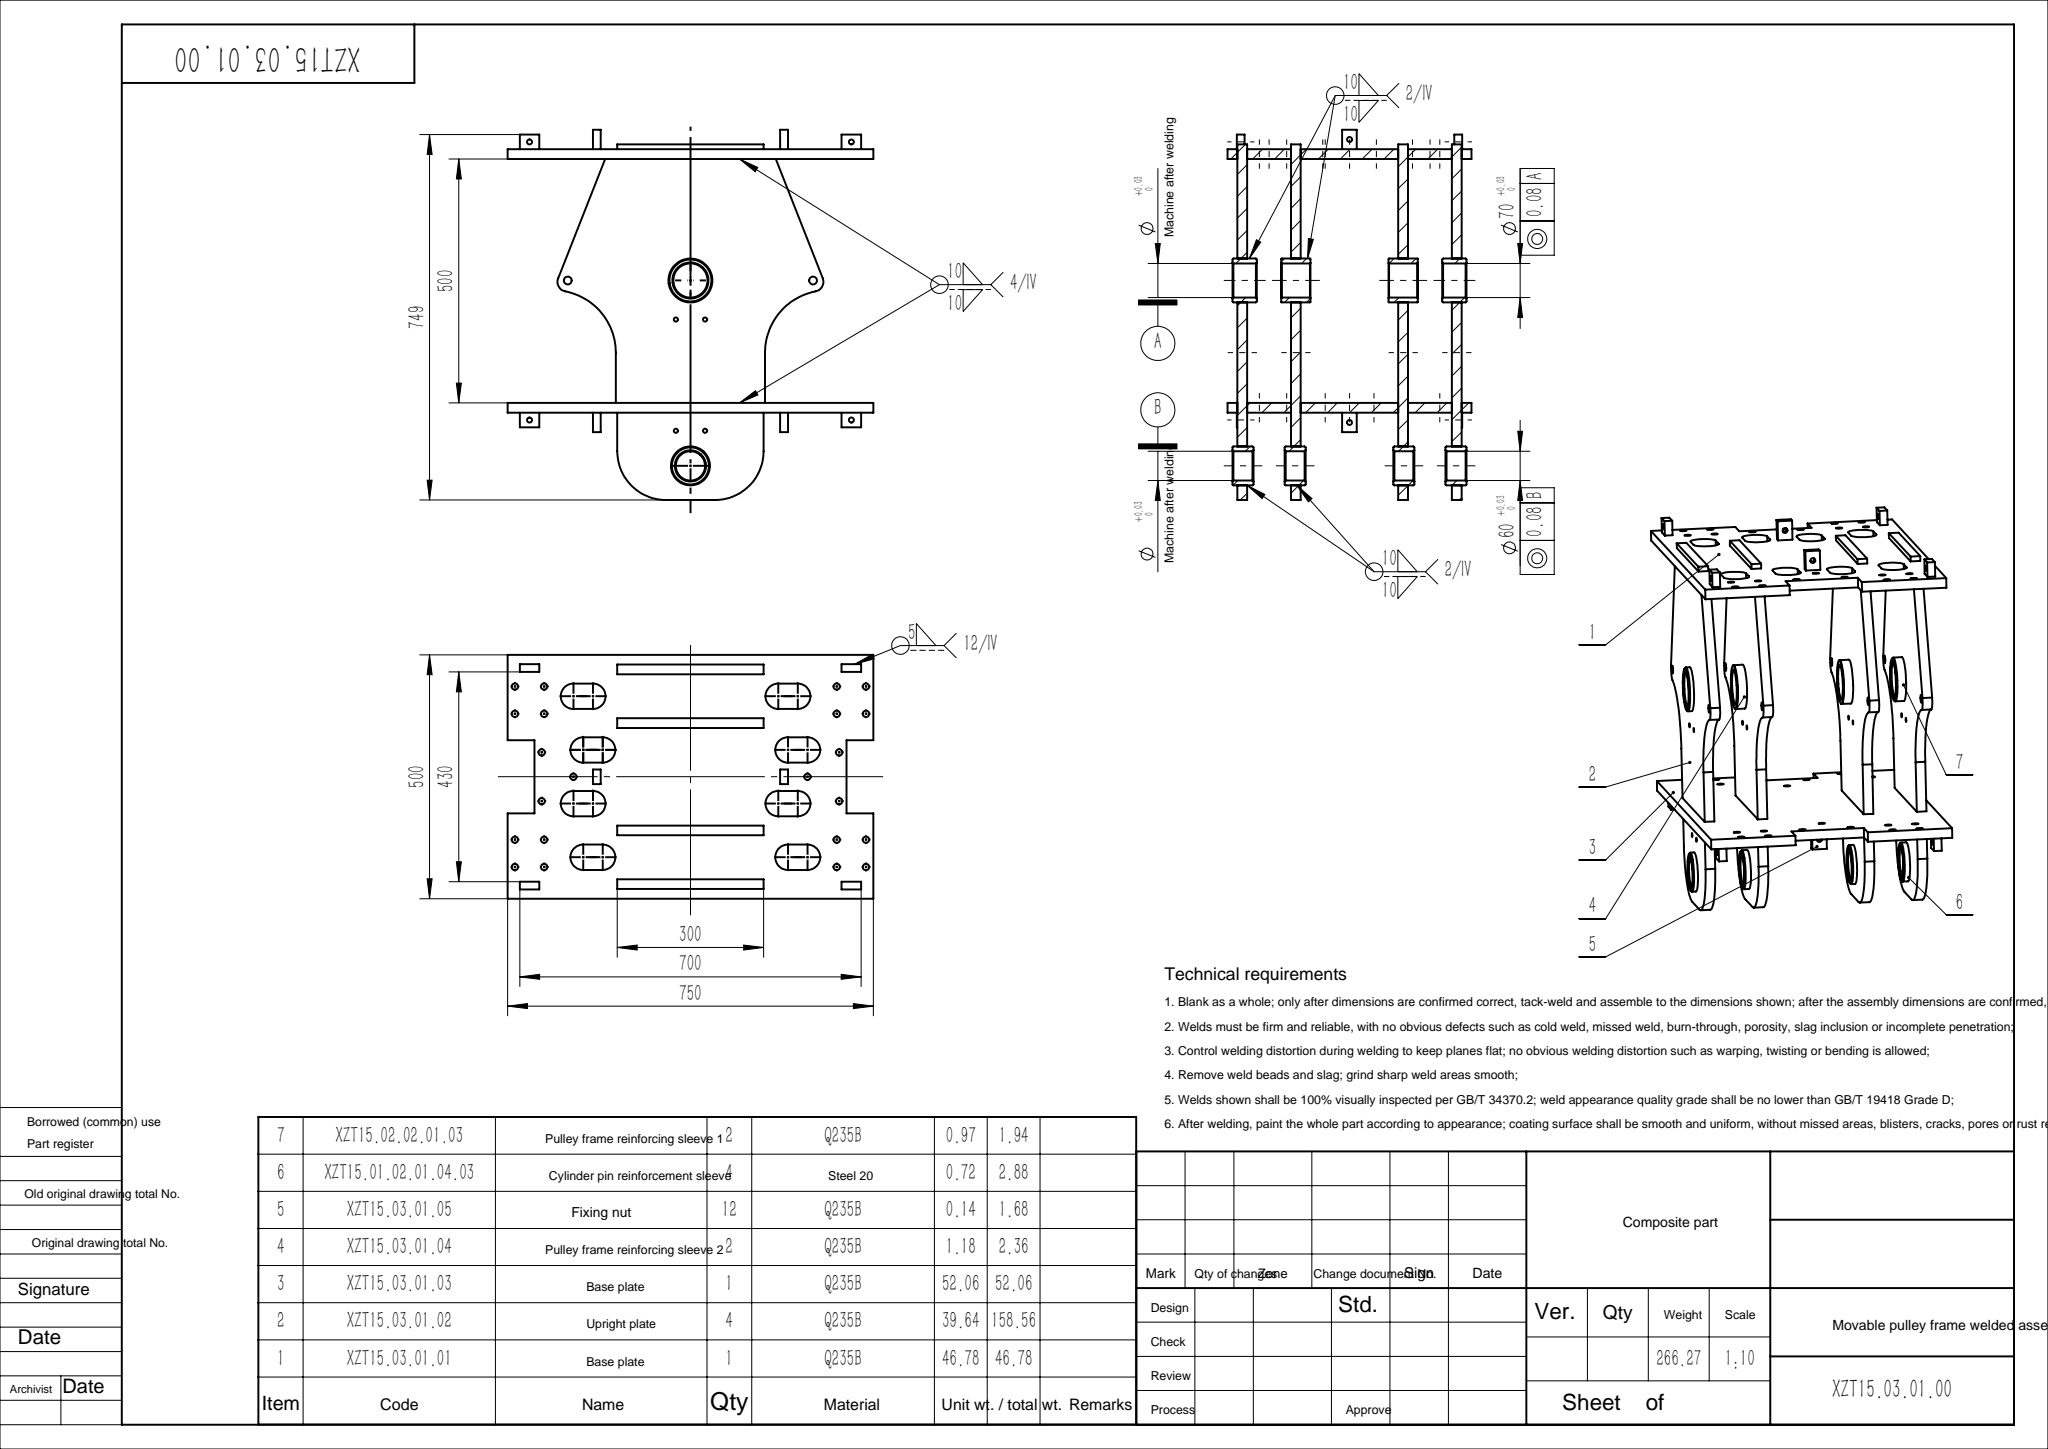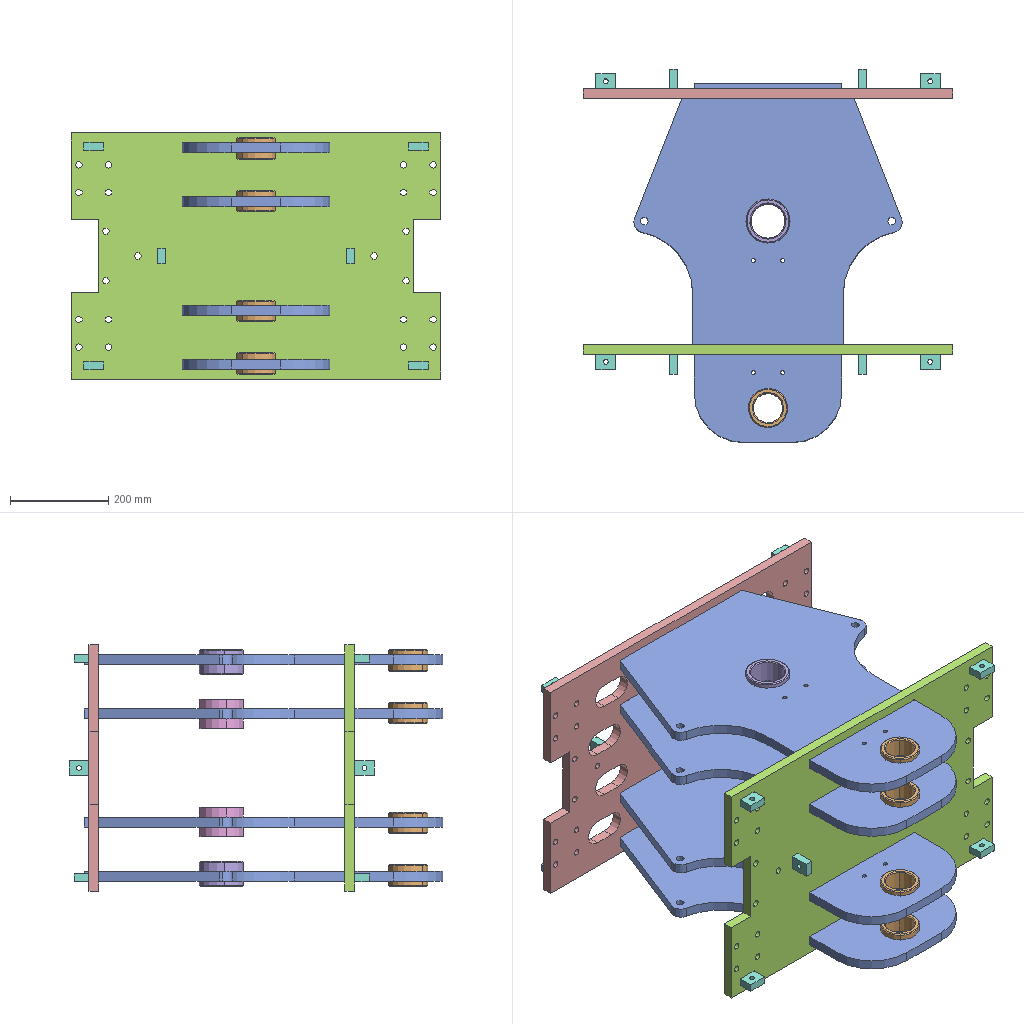Assembly | SolidWorks | 7 different items | 26 placed | box 750 x 759 x 500 mm
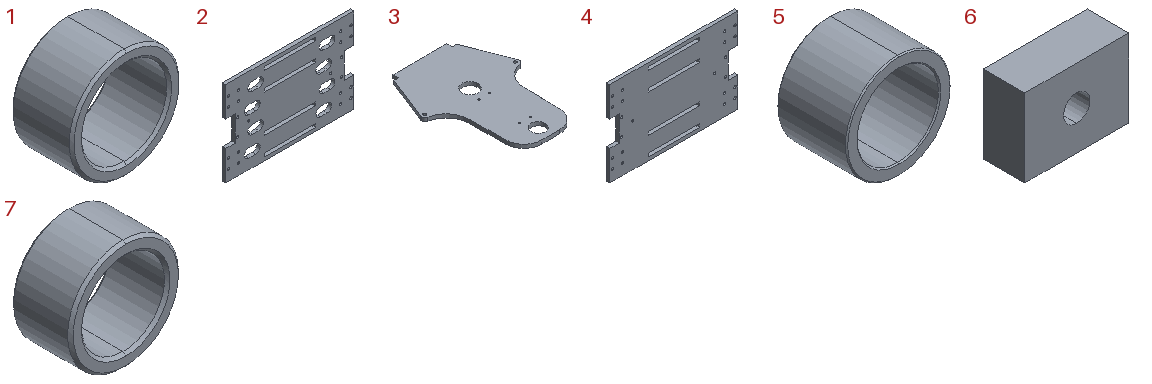Parts list (item | quantity | size | volume | features):
1 | x2 | 90 x 50 x 90 mm | 123653 mm3 | features Chamfer 1, Extrusion 1
2 | x1 | 750 x 20 x 500 mm | 5959003 mm3 | features Extrusion 1, HoleWzd 1, ICE 1
3 | x4 | 545.397 x 729 x 20 mm | 5049504 mm3 | features Fillet 2, Extrusion 1, HoleWzd 1
4 | x1 | 750 x 20 x 500 mm | 6631598 mm3 | features Extrusion 1, HoleWzd 1
5 | x2 | 90 x 60 x 90 mm | 150294 mm3 | features Chamfer 1, Extrusion 1
6 | x12 | 40 x 16 x 30 mm | 17893 mm3 | features Extrusion 1, HoleWzd 1
7 | x4 | 80 x 43 x 80 mm | 92803 mm3 | features Chamfer 1, Extrusion 1
Mates (type | each side: item.copy, entity, surface, feature):
Coordinate | 4.1 select_type:25 | assembly select_type:11
Coincident | 2.1 face plane Boss-Extrude1 | 4.1 face plane Boss-Extrude1 | 2 times
Coincident | 3.1 face plane Boss-Extrude1 | 4.1 face plane Boss-Extrude1 | 3 times
Coincident | 2.1 face plane Boss-Extrude1 | 3.1 face plane Boss-Extrude1
Coincident | 2.1 face plane Boss-Extrude1 | 6.1 face plane Boss-Extrude1
Coincident | 2.1 face plane Boss-Extrude1 | 6.2 face plane Boss-Extrude1
Coincident | 6.2 plane | assembly plane
DistanceDim | 6.1 face plane Boss-Extrude1 | 6.3 face plane Boss-Extrude1
DistanceDim | 6.1 face plane Boss-Extrude1 | 6.4 face plane Boss-Extrude1
DistanceDim | 6.5 face plane Boss-Extrude1 | 6.2 face plane Boss-Extrude1
Coincident | 3.1 face plane Boss-Extrude1 | 3.2 face plane Boss-Extrude1
Coincident | 4.1 face plane Boss-Extrude1 | 3.2 face plane Boss-Extrude1 | 2 times
Concentric | 5.1 face cylinder Boss-Extrude1 | 3.2 face cylinder Boss-Extrude1
Width | 5.1 face plane Boss-Extrude1 | 5.1 face plane Boss-Extrude1 | 3.2 face plane Boss-Extrude1 | 3.2 face plane Boss-Extrude1
Concentric | 3.1 face cylinder Boss-Extrude1 | 7.1 face cylinder Boss-Extrude1
Concentric | 3.2 face cylinder Boss-Extrude1 | 7.2 face cylinder Boss-Extrude1
Concentric | 3.1 face cylinder Boss-Extrude1 | 1.1 face cylinder Boss-Extrude1
DistanceDim | 1.1 face plane Boss-Extrude1 | 3.1 face plane Boss-Extrude1
DistanceDim | 7.1 face plane Boss-Extrude1 | 7.3 face plane Boss-Extrude1
DistanceDim | 7.2 face plane Boss-Extrude1 | 7.4 face plane Boss-Extrude1